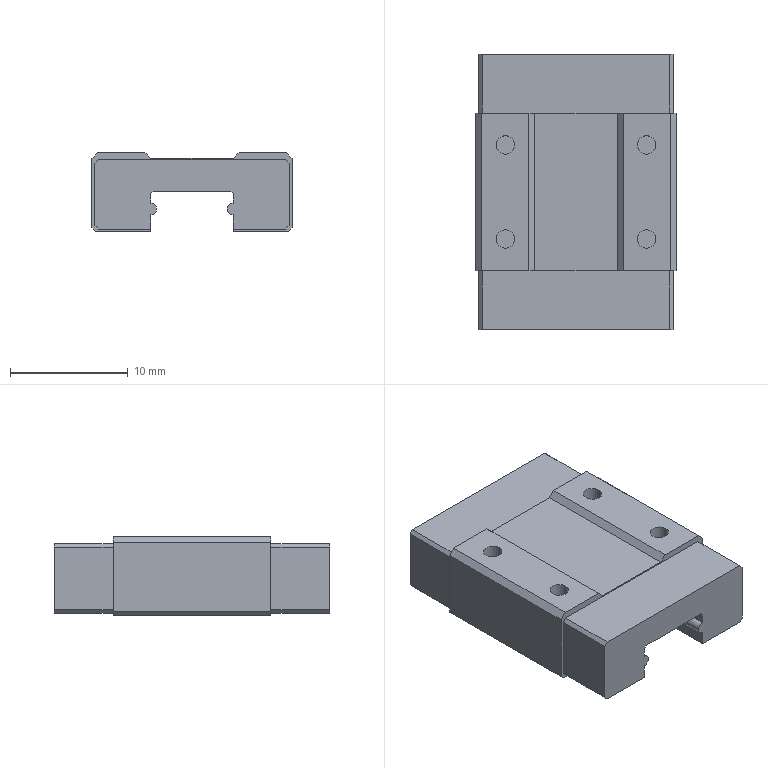Part | SolidWorks | features BaseBody 1 | 1 solid | 57 faces | box 17 x 23.4 x 6.7 mm | volume 1902 mm3 | plane 46 | cylinder 11 | commonest cylinder face diameters 1.567 x8 1 x3